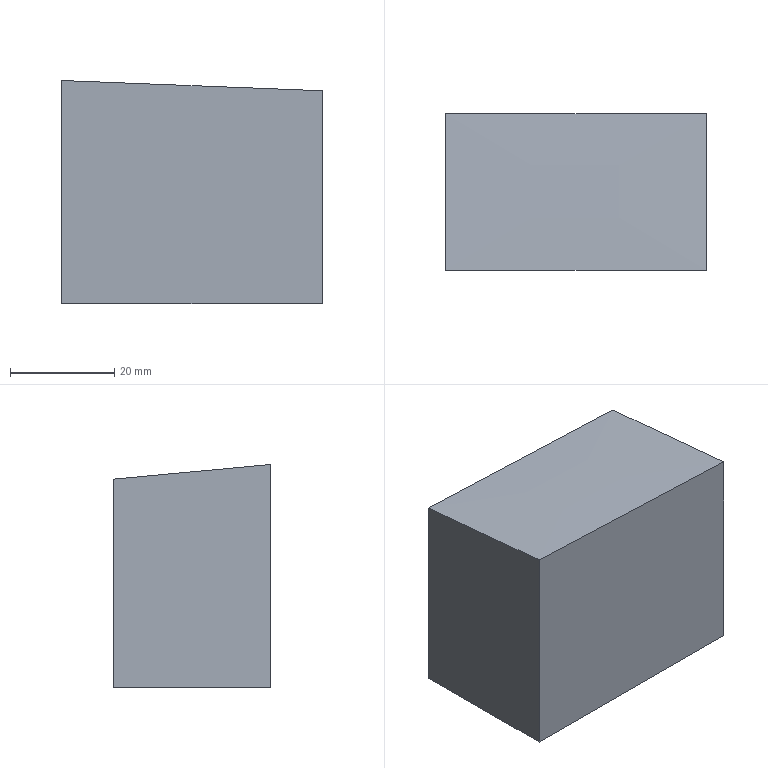Part | NX | features solid 2 | 1 solid | 6 faces | box 50 x 30 x 42.764 mm | volume 60664 mm3 | plane 5 | spline 1
STEP:
#1=CARTESIAN_POINT('',(47.5,375.,74.95));
#2=VERTEX_POINT('',#1);
#3=CARTESIAN_POINT('',(97.5,375.,72.968));
#4=VERTEX_POINT('',#3);
#5=CARTESIAN_POINT('',(47.5,375.,74.95));
#6=CARTESIAN_POINT('',(64.169,375.,74.366));
#7=CARTESIAN_POINT('',(80.837,375.,73.705));
#8=CARTESIAN_POINT('',(97.5,375.,72.968));
#9=B_SPLINE_CURVE_WITH_KNOTS('',3,(#5,#6,#7,#8),.UNSPECIFIED.,.F.,.F.,(4,4),(0.07669,0.1267),.UNSPECIFIED.);
#10=EDGE_CURVE('',#2,#4,#9,.T.);
#11=ORIENTED_EDGE('',*,*,#10,.T.);
#12=CARTESIAN_POINT('',(97.5,375.,35.));
#13=VERTEX_POINT('',#12);
#14=CARTESIAN_POINT('',(97.5,375.,80.));
#15=DIRECTION('',(0.,0.,-1.));
#16=VECTOR('',#15,1000.);
#17=LINE('',#14,#16);
#18=EDGE_CURVE('',#4,#13,#17,.T.);
#19=ORIENTED_EDGE('',*,*,#18,.T.);
#20=CARTESIAN_POINT('',(47.5,375.,35.));
#21=VERTEX_POINT('',#20);
#22=CARTESIAN_POINT('',(47.5,375.,35.));
#23=DIRECTION('',(1.,0.,0.));
#24=VECTOR('',#23,1000.);
#25=LINE('',#22,#24);
#26=EDGE_CURVE('',#21,#13,#25,.T.);
#27=ORIENTED_EDGE('',*,*,#26,.F.);
#28=CARTESIAN_POINT('',(47.5,375.,80.));
#29=DIRECTION('',(0.,0.,-1.));
#30=VECTOR('',#29,1000.);
#31=LINE('',#28,#30);
#32=EDGE_CURVE('',#2,#21,#31,.T.);
#33=ORIENTED_EDGE('',*,*,#32,.F.);
#34=EDGE_LOOP('',(#11,#19,#27,#33));
#35=FACE_BOUND('',#34,.T.);
#36=CARTESIAN_POINT('',(47.5,375.,80.));
#37=DIRECTION('',(0.,-1.,0.));
#38=DIRECTION('',(0.,0.,-1.));
#39=AXIS2_PLACEMENT_3D('',#36,#37,#38);
#40=PLANE('',#39);
#41=ADVANCED_FACE('',(#35),#40,.F.);
#42=CARTESIAN_POINT('',(97.5,345.,75.793));
#43=VERTEX_POINT('',#42);
#44=CARTESIAN_POINT('',(47.5,345.,77.764));
#45=VERTEX_POINT('',#44);
#46=CARTESIAN_POINT('',(97.5,345.,75.793));
#47=CARTESIAN_POINT('',(80.837,345.,76.527));
#48=CARTESIAN_POINT('',(64.169,345.,77.184));
#49=CARTESIAN_POINT('',(47.5,345.,77.764));
#50=B_SPLINE_CURVE_WITH_KNOTS('',3,(#46,#47,#48,#49),.UNSPECIFIED.,.F.,.F.,(4,4),(0.2794,0.3294),.UNSPECIFIED.);
#51=EDGE_CURVE('',#43,#45,#50,.T.);
#52=ORIENTED_EDGE('',*,*,#51,.T.);
#53=CARTESIAN_POINT('',(47.5,345.,35.));
#54=VERTEX_POINT('',#53);
#55=CARTESIAN_POINT('',(47.5,345.,80.));
#56=DIRECTION('',(0.,0.,-1.));
#57=VECTOR('',#56,1000.);
#58=LINE('',#55,#57);
#59=EDGE_CURVE('',#45,#54,#58,.T.);
#60=ORIENTED_EDGE('',*,*,#59,.T.);
#61=CARTESIAN_POINT('',(97.5,345.,35.));
#62=VERTEX_POINT('',#61);
#63=CARTESIAN_POINT('',(415.,345.,35.));
#64=DIRECTION('',(-1.,0.,0.));
#65=VECTOR('',#64,1000.);
#66=LINE('',#63,#65);
#67=EDGE_CURVE('',#54,#62,#66,.F.);
#68=ORIENTED_EDGE('',*,*,#67,.T.);
#69=CARTESIAN_POINT('',(97.5,345.,80.));
#70=DIRECTION('',(0.,0.,-1.));
#71=VECTOR('',#70,1000.);
#72=LINE('',#69,#71);
#73=EDGE_CURVE('',#43,#62,#72,.T.);
#74=ORIENTED_EDGE('',*,*,#73,.F.);
#75=EDGE_LOOP('',(#52,#60,#68,#74));
#76=FACE_BOUND('',#75,.T.);
#77=CARTESIAN_POINT('',(47.5,345.,80.));
#78=DIRECTION('',(0.,-1.,0.));
#79=DIRECTION('',(0.,0.,-1.));
#80=AXIS2_PLACEMENT_3D('',#77,#78,#79);
#81=PLANE('',#80);
#82=ADVANCED_FACE('',(#76),#81,.T.);
#83=ORIENTED_EDGE('',*,*,#32,.T.);
#84=CARTESIAN_POINT('',(47.5,595.,35.));
#85=DIRECTION('',(0.,1.,0.));
#86=VECTOR('',#85,1000.);
#87=LINE('',#84,#86);
#88=EDGE_CURVE('',#21,#54,#87,.F.);
#89=ORIENTED_EDGE('',*,*,#88,.T.);
#90=ORIENTED_EDGE('',*,*,#59,.F.);
#91=CARTESIAN_POINT('',(47.5,375.,74.95));
#92=CARTESIAN_POINT('',(47.5,365.007,75.959));
#93=CARTESIAN_POINT('',(47.5,355.006,76.894));
#94=CARTESIAN_POINT('',(47.5,345.,77.764));
#95=B_SPLINE_CURVE_WITH_KNOTS('',3,(#91,#92,#93,#94),.UNSPECIFIED.,.F.,.F.,(4,4),(0.,0.03013),.UNSPECIFIED.);
#96=EDGE_CURVE('',#2,#45,#95,.T.);
#97=ORIENTED_EDGE('',*,*,#96,.F.);
#98=EDGE_LOOP('',(#83,#89,#90,#97));
#99=FACE_BOUND('',#98,.T.);
#100=CARTESIAN_POINT('',(47.5,375.,80.));
#101=DIRECTION('',(-1.,0.,0.));
#102=DIRECTION('',(0.,0.,-1.));
#103=AXIS2_PLACEMENT_3D('',#100,#101,#102);
#104=PLANE('',#103);
#105=ADVANCED_FACE('',(#99),#104,.T.);
#106=ORIENTED_EDGE('',*,*,#73,.T.);
#107=CARTESIAN_POINT('',(97.5,595.,35.));
#108=DIRECTION('',(0.,1.,0.));
#109=VECTOR('',#108,1000.);
#110=LINE('',#107,#109);
#111=EDGE_CURVE('',#13,#62,#110,.F.);
#112=ORIENTED_EDGE('',*,*,#111,.F.);
#113=ORIENTED_EDGE('',*,*,#18,.F.);
#114=CARTESIAN_POINT('',(97.5,345.,75.793));
#115=CARTESIAN_POINT('',(97.5,355.006,74.92));
#116=CARTESIAN_POINT('',(97.5,365.009,73.981));
#117=CARTESIAN_POINT('',(97.5,375.,72.968));
#118=B_SPLINE_CURVE_WITH_KNOTS('',3,(#114,#115,#116,#117),.UNSPECIFIED.,.F.,.F.,(4,4),(0.1744,0.2045),.UNSPECIFIED.);
#119=EDGE_CURVE('',#43,#4,#118,.T.);
#120=ORIENTED_EDGE('',*,*,#119,.F.);
#121=EDGE_LOOP('',(#106,#112,#113,#120));
#122=FACE_BOUND('',#121,.T.);
#123=CARTESIAN_POINT('',(97.5,375.,80.));
#124=DIRECTION('',(-1.,0.,0.));
#125=DIRECTION('',(0.,0.,-1.));
#126=AXIS2_PLACEMENT_3D('',#123,#124,#125);
#127=PLANE('',#126);
#128=ADVANCED_FACE('',(#122),#127,.F.);
#129=ORIENTED_EDGE('',*,*,#26,.T.);
#130=ORIENTED_EDGE('',*,*,#111,.T.);
#131=ORIENTED_EDGE('',*,*,#67,.F.);
#132=ORIENTED_EDGE('',*,*,#88,.F.);
#133=EDGE_LOOP('',(#129,#130,#131,#132));
#134=FACE_BOUND('',#133,.T.);
#135=CARTESIAN_POINT('',(415.,595.,35.));
#136=DIRECTION('',(0.,0.,1.));
#137=DIRECTION('',(0.,-1.,0.));
#138=AXIS2_PLACEMENT_3D('',#135,#136,#137);
#139=PLANE('',#138);
#140=ADVANCED_FACE('',(#134),#139,.F.);
#141=ORIENTED_EDGE('',*,*,#10,.F.);
#142=ORIENTED_EDGE('',*,*,#96,.T.);
#143=ORIENTED_EDGE('',*,*,#51,.F.);
#144=ORIENTED_EDGE('',*,*,#119,.T.);
#145=EDGE_LOOP('',(#141,#142,#143,#144));
#146=FACE_BOUND('',#145,.T.);
#147=CARTESIAN_POINT('',(47.203,344.816,77.791));
#148=CARTESIAN_POINT('',(63.888,344.817,77.211));
#149=CARTESIAN_POINT('',(80.767,344.818,76.547));
#150=CARTESIAN_POINT('',(97.822,344.818,75.795));
#151=CARTESIAN_POINT('',(47.198,355.05,76.902));
#152=CARTESIAN_POINT('',(63.883,355.051,76.322));
#153=CARTESIAN_POINT('',(80.761,355.052,75.656));
#154=CARTESIAN_POINT('',(97.816,355.052,74.904));
#155=CARTESIAN_POINT('',(47.193,365.171,75.953));
#156=CARTESIAN_POINT('',(63.877,365.172,75.371));
#157=CARTESIAN_POINT('',(80.755,365.172,74.705));
#158=CARTESIAN_POINT('',(97.81,365.173,73.951));
#159=CARTESIAN_POINT('',(47.187,375.178,74.943));
#160=CARTESIAN_POINT('',(63.871,375.179,74.359));
#161=CARTESIAN_POINT('',(80.749,375.18,73.691));
#162=CARTESIAN_POINT('',(97.803,375.18,72.936));
#163=B_SPLINE_SURFACE_WITH_KNOTS('',3,3,((#147,#148,#149,#150),(#151,#152,#153,#154),(#155,#156,#157,#158),(#159,#160,#161,#162)),.UNSPECIFIED.,.F.,.F.,.F.,(4,4),(4,4),(0.6983,0.7626),(0.2833,0.3482),.UNSPECIFIED.);
#164=ADVANCED_FACE('',(#146),#163,.F.);
#165=CLOSED_SHELL('',(#41,#82,#105,#128,#140,#164));
#166=MANIFOLD_SOLID_BREP('',#165);
#167=(LENGTH_UNIT()NAMED_UNIT(*)SI_UNIT(.MILLI.,.METRE.));
#168=UNCERTAINTY_MEASURE_WITH_UNIT(LENGTH_MEASURE(0.0508),#167,'','');
#169=(NAMED_UNIT(*)PLANE_ANGLE_UNIT()SI_UNIT($,.RADIAN.));
#170=(NAMED_UNIT(*)SI_UNIT($,.STERADIAN.)SOLID_ANGLE_UNIT());
#171=(GEOMETRIC_REPRESENTATION_CONTEXT(3)GLOBAL_UNCERTAINTY_ASSIGNED_CONTEXT((#168))GLOBAL_UNIT_ASSIGNED_CONTEXT((#167,#169,#170))REPRESENTATION_CONTEXT('',''));
#172=ADVANCED_BREP_SHAPE_REPRESENTATION('',(#166),#171);